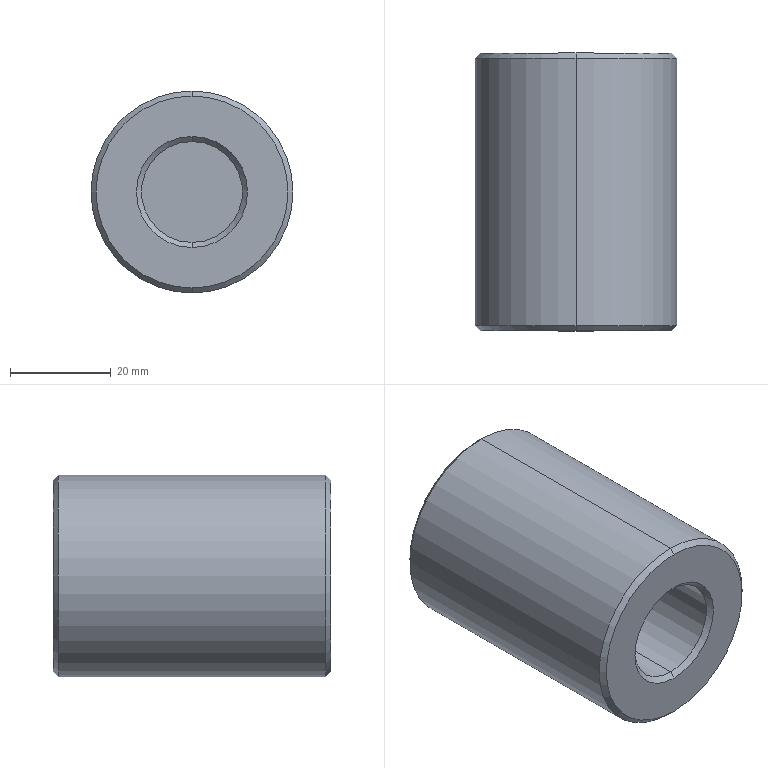Part | SolidWorks | features ICE 2, Chamfer 1, Extrusion 1 | 1 solid | 18 faces | box 40 x 55 x 40 mm | volume 58108 mm3 | cone 8 | cylinder 6 | plane 4 | commonest cylinder face diameters 17 x2 20 x2 40 x2
STEP:
#1=CARTESIAN_POINT('',(0.,0.,-19.));
#2=VERTEX_POINT('',#1);
#3=CARTESIAN_POINT('',(0.,0.,19.));
#4=VERTEX_POINT('',#3);
#5=CARTESIAN_POINT('',(0.,0.,0.));
#6=DIRECTION('',(0.,-1.,0.));
#7=DIRECTION('',(0.,0.,1.));
#8=AXIS2_PLACEMENT_3D('',#5,#6,#7);
#9=CIRCLE('',#8,19.);
#10=EDGE_CURVE('',#2,#4,#9,.T.);
#11=ORIENTED_EDGE('',*,*,#10,.F.);
#12=CARTESIAN_POINT('',(0.,1.,-20.));
#13=VERTEX_POINT('',#12);
#14=CARTESIAN_POINT('',(0.,1.,-20.));
#15=DIRECTION('',(0.,0.7071,-0.7071));
#16=VECTOR('',#15,1000.);
#17=LINE('',#14,#16);
#18=EDGE_CURVE('',#2,#13,#17,.T.);
#19=ORIENTED_EDGE('',*,*,#18,.T.);
#20=CARTESIAN_POINT('',(0.,1.,20.));
#21=VERTEX_POINT('',#20);
#22=CARTESIAN_POINT('',(0.,1.,0.));
#23=DIRECTION('',(0.,1.,0.));
#24=DIRECTION('',(0.,0.,1.));
#25=AXIS2_PLACEMENT_3D('',#22,#23,#24);
#26=CIRCLE('',#25,20.);
#27=EDGE_CURVE('',#21,#13,#26,.T.);
#28=ORIENTED_EDGE('',*,*,#27,.F.);
#29=CARTESIAN_POINT('',(0.,1.,20.));
#30=DIRECTION('',(0.,0.7071,0.7071));
#31=VECTOR('',#30,1000.);
#32=LINE('',#29,#31);
#33=EDGE_CURVE('',#4,#21,#32,.T.);
#34=ORIENTED_EDGE('',*,*,#33,.F.);
#35=EDGE_LOOP('',(#11,#19,#28,#34));
#36=FACE_OUTER_BOUND('',#35,.T.);
#37=CARTESIAN_POINT('',(0.,1.,0.));
#38=DIRECTION('',(0.,1.,0.));
#39=DIRECTION('',(0.,0.,1.));
#40=AXIS2_PLACEMENT_3D('',#37,#38,#39);
#41=CONICAL_SURFACE('',#40,20.,0.7854);
#42=ADVANCED_FACE('',(#36),#41,.T.);
#43=CARTESIAN_POINT('',(0.,55.,19.));
#44=VERTEX_POINT('',#43);
#45=CARTESIAN_POINT('',(0.,55.,-19.));
#46=VERTEX_POINT('',#45);
#47=CARTESIAN_POINT('',(0.,55.,0.));
#48=DIRECTION('',(0.,1.,0.));
#49=DIRECTION('',(0.,0.,1.));
#50=AXIS2_PLACEMENT_3D('',#47,#48,#49);
#51=CIRCLE('',#50,19.);
#52=EDGE_CURVE('',#44,#46,#51,.T.);
#53=ORIENTED_EDGE('',*,*,#52,.F.);
#54=CARTESIAN_POINT('',(0.,54.,20.));
#55=VERTEX_POINT('',#54);
#56=CARTESIAN_POINT('',(0.,55.,19.));
#57=DIRECTION('',(0.,-0.7071,0.7071));
#58=VECTOR('',#57,1000.);
#59=LINE('',#56,#58);
#60=EDGE_CURVE('',#44,#55,#59,.T.);
#61=ORIENTED_EDGE('',*,*,#60,.T.);
#62=CARTESIAN_POINT('',(0.,54.,-20.));
#63=VERTEX_POINT('',#62);
#64=CARTESIAN_POINT('',(0.,54.,0.));
#65=DIRECTION('',(0.,-1.,0.));
#66=DIRECTION('',(0.,0.,1.));
#67=AXIS2_PLACEMENT_3D('',#64,#65,#66);
#68=CIRCLE('',#67,20.);
#69=EDGE_CURVE('',#63,#55,#68,.T.);
#70=ORIENTED_EDGE('',*,*,#69,.F.);
#71=CARTESIAN_POINT('',(0.,55.,-19.));
#72=DIRECTION('',(0.,-0.7071,-0.7071));
#73=VECTOR('',#72,1000.);
#74=LINE('',#71,#73);
#75=EDGE_CURVE('',#46,#63,#74,.T.);
#76=ORIENTED_EDGE('',*,*,#75,.F.);
#77=EDGE_LOOP('',(#53,#61,#70,#76));
#78=FACE_OUTER_BOUND('',#77,.T.);
#79=CARTESIAN_POINT('',(0.,55.,0.));
#80=DIRECTION('',(0.,-1.,0.));
#81=DIRECTION('',(0.,0.,-1.));
#82=AXIS2_PLACEMENT_3D('',#79,#80,#81);
#83=CONICAL_SURFACE('',#82,19.,0.7854);
#84=ADVANCED_FACE('',(#78),#83,.T.);
#85=CARTESIAN_POINT('',(0.,1.,10.));
#86=VERTEX_POINT('',#85);
#87=CARTESIAN_POINT('',(0.,1.,-10.));
#88=VERTEX_POINT('',#87);
#89=CARTESIAN_POINT('',(0.,1.,0.));
#90=DIRECTION('',(0.,-1.,0.));
#91=DIRECTION('',(0.,0.,1.));
#92=AXIS2_PLACEMENT_3D('',#89,#90,#91);
#93=CIRCLE('',#92,10.);
#94=EDGE_CURVE('',#86,#88,#93,.T.);
#95=ORIENTED_EDGE('',*,*,#94,.F.);
#96=CARTESIAN_POINT('',(0.,0.,11.));
#97=VERTEX_POINT('',#96);
#98=CARTESIAN_POINT('',(0.,1.,10.));
#99=DIRECTION('',(0.,-0.7071,0.7071));
#100=VECTOR('',#99,1000.);
#101=LINE('',#98,#100);
#102=EDGE_CURVE('',#86,#97,#101,.T.);
#103=ORIENTED_EDGE('',*,*,#102,.T.);
#104=CARTESIAN_POINT('',(0.,0.,-11.));
#105=VERTEX_POINT('',#104);
#106=CARTESIAN_POINT('',(0.,0.,0.));
#107=DIRECTION('',(0.,1.,0.));
#108=DIRECTION('',(0.,0.,1.));
#109=AXIS2_PLACEMENT_3D('',#106,#107,#108);
#110=CIRCLE('',#109,11.);
#111=EDGE_CURVE('',#105,#97,#110,.T.);
#112=ORIENTED_EDGE('',*,*,#111,.F.);
#113=CARTESIAN_POINT('',(0.,1.,-10.));
#114=DIRECTION('',(0.,-0.7071,-0.7071));
#115=VECTOR('',#114,1000.);
#116=LINE('',#113,#115);
#117=EDGE_CURVE('',#88,#105,#116,.T.);
#118=ORIENTED_EDGE('',*,*,#117,.F.);
#119=EDGE_LOOP('',(#95,#103,#112,#118));
#120=FACE_OUTER_BOUND('',#119,.T.);
#121=CARTESIAN_POINT('',(0.,1.,0.));
#122=DIRECTION('',(0.,-1.,0.));
#123=DIRECTION('',(0.,0.,-1.));
#124=AXIS2_PLACEMENT_3D('',#121,#122,#123);
#125=CONICAL_SURFACE('',#124,10.,0.7854);
#126=ADVANCED_FACE('',(#120),#125,.F.);
#127=CARTESIAN_POINT('',(0.,54.,-8.5));
#128=VERTEX_POINT('',#127);
#129=CARTESIAN_POINT('',(0.,54.,8.5));
#130=VERTEX_POINT('',#129);
#131=CARTESIAN_POINT('',(0.,54.,0.));
#132=DIRECTION('',(0.,1.,0.));
#133=DIRECTION('',(0.,0.,1.));
#134=AXIS2_PLACEMENT_3D('',#131,#132,#133);
#135=CIRCLE('',#134,8.5);
#136=EDGE_CURVE('',#128,#130,#135,.T.);
#137=ORIENTED_EDGE('',*,*,#136,.F.);
#138=CARTESIAN_POINT('',(0.,55.,-9.5));
#139=VERTEX_POINT('',#138);
#140=CARTESIAN_POINT('',(0.,54.,-8.5));
#141=DIRECTION('',(0.,0.7071,-0.7071));
#142=VECTOR('',#141,1000.);
#143=LINE('',#140,#142);
#144=EDGE_CURVE('',#128,#139,#143,.T.);
#145=ORIENTED_EDGE('',*,*,#144,.T.);
#146=CARTESIAN_POINT('',(0.,55.,9.5));
#147=VERTEX_POINT('',#146);
#148=CARTESIAN_POINT('',(0.,55.,0.));
#149=DIRECTION('',(0.,-1.,0.));
#150=DIRECTION('',(0.,0.,1.));
#151=AXIS2_PLACEMENT_3D('',#148,#149,#150);
#152=CIRCLE('',#151,9.5);
#153=EDGE_CURVE('',#147,#139,#152,.T.);
#154=ORIENTED_EDGE('',*,*,#153,.F.);
#155=CARTESIAN_POINT('',(0.,54.,8.5));
#156=DIRECTION('',(0.,0.7071,0.7071));
#157=VECTOR('',#156,1000.);
#158=LINE('',#155,#157);
#159=EDGE_CURVE('',#130,#147,#158,.T.);
#160=ORIENTED_EDGE('',*,*,#159,.F.);
#161=EDGE_LOOP('',(#137,#145,#154,#160));
#162=FACE_OUTER_BOUND('',#161,.T.);
#163=CARTESIAN_POINT('',(0.,54.,0.));
#164=DIRECTION('',(0.,1.,0.));
#165=DIRECTION('',(0.,0.,1.));
#166=AXIS2_PLACEMENT_3D('',#163,#164,#165);
#167=CONICAL_SURFACE('',#166,8.5,0.7854);
#168=ADVANCED_FACE('',(#162),#167,.F.);
#169=CARTESIAN_POINT('',(0.,20.,10.));
#170=VERTEX_POINT('',#169);
#171=CARTESIAN_POINT('',(0.,20.,-10.));
#172=VERTEX_POINT('',#171);
#173=CARTESIAN_POINT('',(0.,20.,0.));
#174=DIRECTION('',(0.,-1.,0.));
#175=DIRECTION('',(0.,0.,-1.));
#176=AXIS2_PLACEMENT_3D('',#173,#174,#175);
#177=CIRCLE('',#176,10.);
#178=EDGE_CURVE('',#170,#172,#177,.T.);
#179=ORIENTED_EDGE('',*,*,#178,.F.);
#180=CARTESIAN_POINT('',(0.,20.,10.));
#181=DIRECTION('',(0.,-1.,0.));
#182=VECTOR('',#181,1000.);
#183=LINE('',#180,#182);
#184=EDGE_CURVE('',#170,#86,#183,.T.);
#185=ORIENTED_EDGE('',*,*,#184,.T.);
#186=ORIENTED_EDGE('',*,*,#94,.T.);
#187=CARTESIAN_POINT('',(0.,20.,-10.));
#188=DIRECTION('',(0.,-1.,0.));
#189=VECTOR('',#188,1000.);
#190=LINE('',#187,#189);
#191=EDGE_CURVE('',#172,#88,#190,.T.);
#192=ORIENTED_EDGE('',*,*,#191,.F.);
#193=EDGE_LOOP('',(#179,#185,#186,#192));
#194=FACE_OUTER_BOUND('',#193,.T.);
#195=CARTESIAN_POINT('',(0.,20.,0.));
#196=DIRECTION('',(0.,-1.,0.));
#197=DIRECTION('',(0.,0.,-1.));
#198=AXIS2_PLACEMENT_3D('',#195,#196,#197);
#199=CYLINDRICAL_SURFACE('',#198,10.);
#200=ADVANCED_FACE('',(#194),#199,.F.);
#201=CARTESIAN_POINT('',(0.,35.,-8.5));
#202=VERTEX_POINT('',#201);
#203=CARTESIAN_POINT('',(0.,35.,8.5));
#204=VERTEX_POINT('',#203);
#205=CARTESIAN_POINT('',(0.,35.,0.));
#206=DIRECTION('',(0.,1.,0.));
#207=DIRECTION('',(0.,0.,1.));
#208=AXIS2_PLACEMENT_3D('',#205,#206,#207);
#209=CIRCLE('',#208,8.5);
#210=EDGE_CURVE('',#202,#204,#209,.T.);
#211=ORIENTED_EDGE('',*,*,#210,.F.);
#212=CARTESIAN_POINT('',(0.,35.,-8.5));
#213=DIRECTION('',(0.,1.,0.));
#214=VECTOR('',#213,1000.);
#215=LINE('',#212,#214);
#216=EDGE_CURVE('',#202,#128,#215,.T.);
#217=ORIENTED_EDGE('',*,*,#216,.T.);
#218=ORIENTED_EDGE('',*,*,#136,.T.);
#219=CARTESIAN_POINT('',(0.,35.,8.5));
#220=DIRECTION('',(0.,1.,0.));
#221=VECTOR('',#220,1000.);
#222=LINE('',#219,#221);
#223=EDGE_CURVE('',#204,#130,#222,.T.);
#224=ORIENTED_EDGE('',*,*,#223,.F.);
#225=EDGE_LOOP('',(#211,#217,#218,#224));
#226=FACE_OUTER_BOUND('',#225,.T.);
#227=CARTESIAN_POINT('',(0.,35.,0.));
#228=DIRECTION('',(0.,1.,0.));
#229=DIRECTION('',(0.,0.,1.));
#230=AXIS2_PLACEMENT_3D('',#227,#228,#229);
#231=CYLINDRICAL_SURFACE('',#230,8.5);
#232=ADVANCED_FACE('',(#226),#231,.F.);
#233=ORIENTED_EDGE('',*,*,#69,.T.);
#234=CARTESIAN_POINT('',(0.,55.,20.));
#235=DIRECTION('',(0.,-1.,0.));
#236=VECTOR('',#235,1000.);
#237=LINE('',#234,#236);
#238=EDGE_CURVE('',#55,#21,#237,.T.);
#239=ORIENTED_EDGE('',*,*,#238,.T.);
#240=ORIENTED_EDGE('',*,*,#27,.T.);
#241=CARTESIAN_POINT('',(0.,55.,-20.));
#242=DIRECTION('',(0.,-1.,0.));
#243=VECTOR('',#242,1000.);
#244=LINE('',#241,#243);
#245=EDGE_CURVE('',#63,#13,#244,.T.);
#246=ORIENTED_EDGE('',*,*,#245,.F.);
#247=EDGE_LOOP('',(#233,#239,#240,#246));
#248=FACE_OUTER_BOUND('',#247,.T.);
#249=CARTESIAN_POINT('',(0.,55.,0.));
#250=DIRECTION('',(0.,-1.,0.));
#251=DIRECTION('',(0.,0.,-1.));
#252=AXIS2_PLACEMENT_3D('',#249,#250,#251);
#253=CYLINDRICAL_SURFACE('',#252,20.);
#254=ADVANCED_FACE('',(#248),#253,.T.);
#255=ORIENTED_EDGE('',*,*,#238,.F.);
#256=CARTESIAN_POINT('',(0.,54.,0.));
#257=DIRECTION('',(0.,-1.,0.));
#258=DIRECTION('',(0.,0.,1.));
#259=AXIS2_PLACEMENT_3D('',#256,#257,#258);
#260=CIRCLE('',#259,20.);
#261=EDGE_CURVE('',#55,#63,#260,.T.);
#262=ORIENTED_EDGE('',*,*,#261,.T.);
#263=ORIENTED_EDGE('',*,*,#245,.T.);
#264=CARTESIAN_POINT('',(0.,1.,0.));
#265=DIRECTION('',(0.,1.,0.));
#266=DIRECTION('',(0.,0.,1.));
#267=AXIS2_PLACEMENT_3D('',#264,#265,#266);
#268=CIRCLE('',#267,20.);
#269=EDGE_CURVE('',#13,#21,#268,.T.);
#270=ORIENTED_EDGE('',*,*,#269,.T.);
#271=EDGE_LOOP('',(#255,#262,#263,#270));
#272=FACE_OUTER_BOUND('',#271,.T.);
#273=CARTESIAN_POINT('',(0.,55.,0.));
#274=DIRECTION('',(0.,-1.,0.));
#275=DIRECTION('',(0.,0.,-1.));
#276=AXIS2_PLACEMENT_3D('',#273,#274,#275);
#277=CYLINDRICAL_SURFACE('',#276,20.);
#278=ADVANCED_FACE('',(#272),#277,.T.);
#279=ORIENTED_EDGE('',*,*,#153,.T.);
#280=CARTESIAN_POINT('',(0.,55.,0.));
#281=DIRECTION('',(0.,-1.,0.));
#282=DIRECTION('',(0.,0.,1.));
#283=AXIS2_PLACEMENT_3D('',#280,#281,#282);
#284=CIRCLE('',#283,9.5);
#285=EDGE_CURVE('',#139,#147,#284,.T.);
#286=ORIENTED_EDGE('',*,*,#285,.T.);
#287=EDGE_LOOP('',(#279,#286));
#288=FACE_BOUND('',#287,.T.);
#289=CARTESIAN_POINT('',(0.,55.,0.));
#290=DIRECTION('',(0.,1.,0.));
#291=DIRECTION('',(0.,0.,1.));
#292=AXIS2_PLACEMENT_3D('',#289,#290,#291);
#293=CIRCLE('',#292,19.);
#294=EDGE_CURVE('',#46,#44,#293,.T.);
#295=ORIENTED_EDGE('',*,*,#294,.T.);
#296=ORIENTED_EDGE('',*,*,#52,.T.);
#297=EDGE_LOOP('',(#295,#296));
#298=FACE_OUTER_BOUND('',#297,.T.);
#299=CARTESIAN_POINT('',(0.,55.,0.));
#300=DIRECTION('',(0.,1.,0.));
#301=DIRECTION('',(0.,0.,1.));
#302=AXIS2_PLACEMENT_3D('',#299,#300,#301);
#303=PLANE('',#302);
#304=ADVANCED_FACE('',(#288,#298),#303,.T.);
#305=ORIENTED_EDGE('',*,*,#111,.T.);
#306=CARTESIAN_POINT('',(0.,0.,0.));
#307=DIRECTION('',(0.,1.,0.));
#308=DIRECTION('',(0.,0.,1.));
#309=AXIS2_PLACEMENT_3D('',#306,#307,#308);
#310=CIRCLE('',#309,11.);
#311=EDGE_CURVE('',#97,#105,#310,.T.);
#312=ORIENTED_EDGE('',*,*,#311,.T.);
#313=EDGE_LOOP('',(#305,#312));
#314=FACE_BOUND('',#313,.T.);
#315=CARTESIAN_POINT('',(0.,0.,0.));
#316=DIRECTION('',(0.,-1.,0.));
#317=DIRECTION('',(0.,0.,1.));
#318=AXIS2_PLACEMENT_3D('',#315,#316,#317);
#319=CIRCLE('',#318,19.);
#320=EDGE_CURVE('',#4,#2,#319,.T.);
#321=ORIENTED_EDGE('',*,*,#320,.T.);
#322=ORIENTED_EDGE('',*,*,#10,.T.);
#323=EDGE_LOOP('',(#321,#322));
#324=FACE_OUTER_BOUND('',#323,.T.);
#325=CARTESIAN_POINT('',(0.,0.,0.));
#326=DIRECTION('',(0.,1.,0.));
#327=DIRECTION('',(0.,0.,1.));
#328=AXIS2_PLACEMENT_3D('',#325,#326,#327);
#329=PLANE('',#328);
#330=ADVANCED_FACE('',(#314,#324),#329,.F.);
#331=ORIENTED_EDGE('',*,*,#216,.F.);
#332=CARTESIAN_POINT('',(0.,35.,0.));
#333=DIRECTION('',(0.,1.,0.));
#334=DIRECTION('',(0.,0.,1.));
#335=AXIS2_PLACEMENT_3D('',#332,#333,#334);
#336=CIRCLE('',#335,8.5);
#337=EDGE_CURVE('',#204,#202,#336,.T.);
#338=ORIENTED_EDGE('',*,*,#337,.F.);
#339=ORIENTED_EDGE('',*,*,#223,.T.);
#340=CARTESIAN_POINT('',(0.,54.,0.));
#341=DIRECTION('',(0.,1.,0.));
#342=DIRECTION('',(0.,0.,1.));
#343=AXIS2_PLACEMENT_3D('',#340,#341,#342);
#344=CIRCLE('',#343,8.5);
#345=EDGE_CURVE('',#130,#128,#344,.T.);
#346=ORIENTED_EDGE('',*,*,#345,.T.);
#347=EDGE_LOOP('',(#331,#338,#339,#346));
#348=FACE_OUTER_BOUND('',#347,.T.);
#349=CARTESIAN_POINT('',(0.,35.,0.));
#350=DIRECTION('',(0.,1.,0.));
#351=DIRECTION('',(0.,0.,1.));
#352=AXIS2_PLACEMENT_3D('',#349,#350,#351);
#353=CYLINDRICAL_SURFACE('',#352,8.5);
#354=ADVANCED_FACE('',(#348),#353,.F.);
#355=ORIENTED_EDGE('',*,*,#337,.T.);
#356=ORIENTED_EDGE('',*,*,#210,.T.);
#357=EDGE_LOOP('',(#355,#356));
#358=FACE_OUTER_BOUND('',#357,.T.);
#359=CARTESIAN_POINT('',(0.,35.,0.));
#360=DIRECTION('',(0.,1.,0.));
#361=DIRECTION('',(0.,0.,1.));
#362=AXIS2_PLACEMENT_3D('',#359,#360,#361);
#363=PLANE('',#362);
#364=ADVANCED_FACE('',(#358),#363,.T.);
#365=ORIENTED_EDGE('',*,*,#184,.F.);
#366=CARTESIAN_POINT('',(0.,20.,0.));
#367=DIRECTION('',(0.,-1.,0.));
#368=DIRECTION('',(0.,0.,-1.));
#369=AXIS2_PLACEMENT_3D('',#366,#367,#368);
#370=CIRCLE('',#369,10.);
#371=EDGE_CURVE('',#172,#170,#370,.T.);
#372=ORIENTED_EDGE('',*,*,#371,.F.);
#373=ORIENTED_EDGE('',*,*,#191,.T.);
#374=CARTESIAN_POINT('',(0.,1.,0.));
#375=DIRECTION('',(0.,-1.,0.));
#376=DIRECTION('',(0.,0.,1.));
#377=AXIS2_PLACEMENT_3D('',#374,#375,#376);
#378=CIRCLE('',#377,10.);
#379=EDGE_CURVE('',#88,#86,#378,.T.);
#380=ORIENTED_EDGE('',*,*,#379,.T.);
#381=EDGE_LOOP('',(#365,#372,#373,#380));
#382=FACE_OUTER_BOUND('',#381,.T.);
#383=CARTESIAN_POINT('',(0.,20.,0.));
#384=DIRECTION('',(0.,-1.,0.));
#385=DIRECTION('',(0.,0.,-1.));
#386=AXIS2_PLACEMENT_3D('',#383,#384,#385);
#387=CYLINDRICAL_SURFACE('',#386,10.);
#388=ADVANCED_FACE('',(#382),#387,.F.);
#389=ORIENTED_EDGE('',*,*,#371,.T.);
#390=ORIENTED_EDGE('',*,*,#178,.T.);
#391=EDGE_LOOP('',(#389,#390));
#392=FACE_OUTER_BOUND('',#391,.T.);
#393=CARTESIAN_POINT('',(0.,20.,0.));
#394=DIRECTION('',(0.,-1.,0.));
#395=DIRECTION('',(0.,0.,-1.));
#396=AXIS2_PLACEMENT_3D('',#393,#394,#395);
#397=PLANE('',#396);
#398=ADVANCED_FACE('',(#392),#397,.T.);
#399=ORIENTED_EDGE('',*,*,#144,.F.);
#400=ORIENTED_EDGE('',*,*,#345,.F.);
#401=ORIENTED_EDGE('',*,*,#159,.T.);
#402=ORIENTED_EDGE('',*,*,#285,.F.);
#403=EDGE_LOOP('',(#399,#400,#401,#402));
#404=FACE_OUTER_BOUND('',#403,.T.);
#405=CARTESIAN_POINT('',(0.,54.,0.));
#406=DIRECTION('',(0.,1.,0.));
#407=DIRECTION('',(0.,0.,1.));
#408=AXIS2_PLACEMENT_3D('',#405,#406,#407);
#409=CONICAL_SURFACE('',#408,8.5,0.7854);
#410=ADVANCED_FACE('',(#404),#409,.F.);
#411=ORIENTED_EDGE('',*,*,#102,.F.);
#412=ORIENTED_EDGE('',*,*,#379,.F.);
#413=ORIENTED_EDGE('',*,*,#117,.T.);
#414=ORIENTED_EDGE('',*,*,#311,.F.);
#415=EDGE_LOOP('',(#411,#412,#413,#414));
#416=FACE_OUTER_BOUND('',#415,.T.);
#417=CARTESIAN_POINT('',(0.,1.,0.));
#418=DIRECTION('',(0.,-1.,0.));
#419=DIRECTION('',(0.,0.,-1.));
#420=AXIS2_PLACEMENT_3D('',#417,#418,#419);
#421=CONICAL_SURFACE('',#420,10.,0.7854);
#422=ADVANCED_FACE('',(#416),#421,.F.);
#423=ORIENTED_EDGE('',*,*,#60,.F.);
#424=ORIENTED_EDGE('',*,*,#294,.F.);
#425=ORIENTED_EDGE('',*,*,#75,.T.);
#426=ORIENTED_EDGE('',*,*,#261,.F.);
#427=EDGE_LOOP('',(#423,#424,#425,#426));
#428=FACE_OUTER_BOUND('',#427,.T.);
#429=CARTESIAN_POINT('',(0.,55.,0.));
#430=DIRECTION('',(0.,-1.,0.));
#431=DIRECTION('',(0.,0.,-1.));
#432=AXIS2_PLACEMENT_3D('',#429,#430,#431);
#433=CONICAL_SURFACE('',#432,19.,0.7854);
#434=ADVANCED_FACE('',(#428),#433,.T.);
#435=ORIENTED_EDGE('',*,*,#18,.F.);
#436=ORIENTED_EDGE('',*,*,#320,.F.);
#437=ORIENTED_EDGE('',*,*,#33,.T.);
#438=ORIENTED_EDGE('',*,*,#269,.F.);
#439=EDGE_LOOP('',(#435,#436,#437,#438));
#440=FACE_OUTER_BOUND('',#439,.T.);
#441=CARTESIAN_POINT('',(0.,1.,0.));
#442=DIRECTION('',(0.,1.,0.));
#443=DIRECTION('',(0.,0.,1.));
#444=AXIS2_PLACEMENT_3D('',#441,#442,#443);
#445=CONICAL_SURFACE('',#444,20.,0.7854);
#446=ADVANCED_FACE('',(#440),#445,.T.);
#447=CLOSED_SHELL('',(#42,#84,#126,#168,#200,#232,#254,#278,#304,#330,#354,#364,#388,#398,#410,#422,#434,#446));
#448=MANIFOLD_SOLID_BREP('',#447);
#449=CARTESIAN_POINT('',(0.,0.,0.));
#450=DIRECTION('',(0.,0.,1.));
#451=DIRECTION('',(1.,0.,0.));
#452=AXIS2_PLACEMENT_3D('',#449,#450,#451);
#453=(LENGTH_UNIT()NAMED_UNIT(*)SI_UNIT(.MILLI.,.METRE.));
#454=UNCERTAINTY_MEASURE_WITH_UNIT(LENGTH_MEASURE(0.00001),#453,'','');
#455=(NAMED_UNIT(*)PLANE_ANGLE_UNIT()SI_UNIT($,.RADIAN.));
#456=(NAMED_UNIT(*)SI_UNIT($,.STERADIAN.)SOLID_ANGLE_UNIT());
#457=(GEOMETRIC_REPRESENTATION_CONTEXT(3)GLOBAL_UNCERTAINTY_ASSIGNED_CONTEXT((#454))GLOBAL_UNIT_ASSIGNED_CONTEXT((#453,#455,#456))REPRESENTATION_CONTEXT('',''));
#458=ADVANCED_BREP_SHAPE_REPRESENTATION('',(#448,#452),#457);